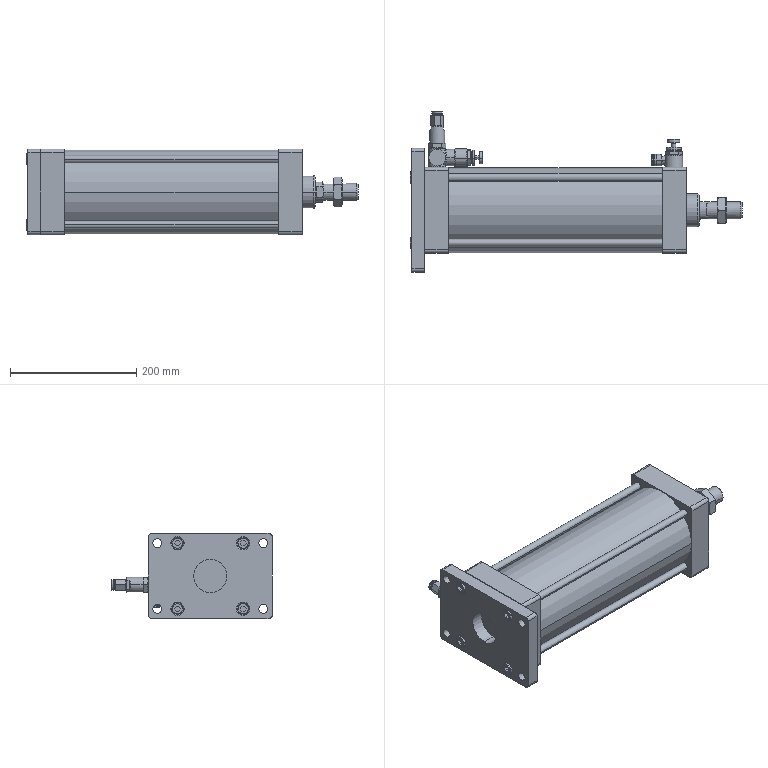Part | SolidWorks | features BaseBody 8 | 8 solids | 714 faces | box 526 x 254 x 136 mm | volume 3520459 mm3 | plane 291 | cylinder 224 | cone 157 | spline 42 | commonest cylinder face diameters 19.2 x24 10 x18 10.106 x16 12 x16 18 x12 6 x8